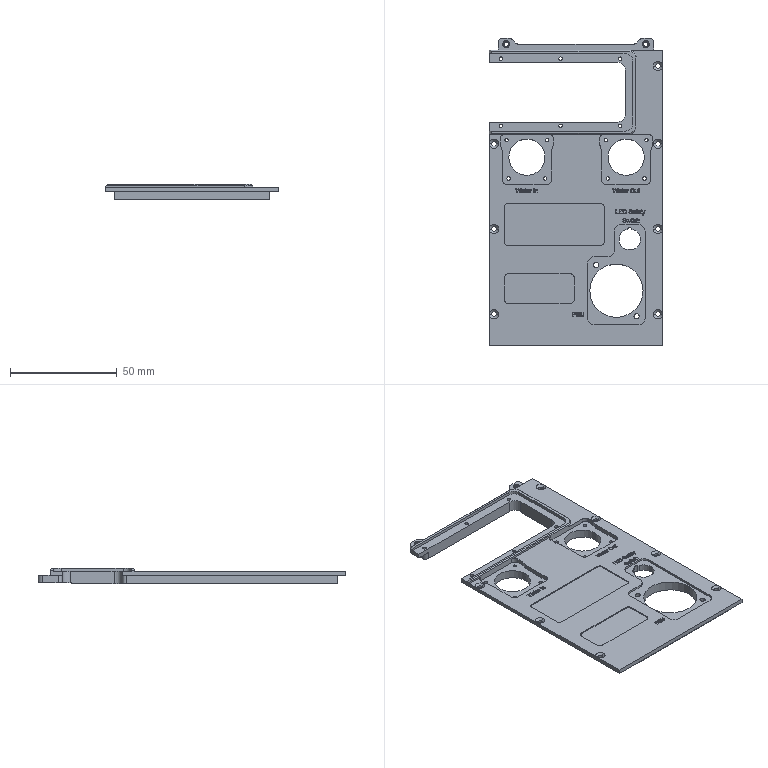NC program | NX | posted with a generic post | part box 81.5 x 144.28 x 7.5 mm
Lines 1 to 2085 of 3119, first 1845 of 2067 lines:
N10 G17 G21 G94 G90
(FLOOR_FACING_COPY , TOOL : D63面刀)
N12 T11 M6
N14 G54
N16 G17 G0 G90 X-113.64 Y25. S4500 M3
N18 G43 Z50. H11
N20 Z5.275
N22 G94 G1 Z2.275 F800.
N24 X-103.64
N26 X103.64
N28 Y-15.55
N30 X-103.64
N32 X-113.64
N34 Z5.275
N36 G0 Z50.
N38 Y25.
N40 Z4.55
N42 G1 Z1.55
N44 X-103.64
N46 X103.64
N48 Y-15.55
N50 X-103.64
N52 X-113.64
N54 Z4.55
N56 G0 Z50.
N58 Y25.
N60 Z3.825
N62 G1 Z0.825
N64 X-103.64
N66 X103.64
N68 Y-15.55
N70 X-103.64
N72 X-113.64
N74 Z3.825
N76 G0 Z50.
N78 Y25.
N80 Z3.1
N82 G1 Z0.1
N84 X-103.64
N86 X103.64
N88 Y-15.55
N90 X-103.64
N92 X-113.64
N94 Z3.1
N96 G0 Z50.
N98 M5
(CAVITY_MILL_COPY_2 , TOOL : D6开粗)
N100 T01 M6
N102 G54
N104 G17 G0 G90 X21.572 Y-44.35 S6500 M3
N106 G43 Z50. H1
N108 Z0.05
N110 G94 G1 Z-0.45 F2500.
N112 Y-41.65
N114 G3 X20.972 Y-41.05 R0.6
N116 G1 X-22.953 Y-41.049
N118 G2 X-24.802 Y-43.749 R4.206
N120 G1 X-30.848
N122 G2 X-32.725 Y-41.049 R4.261
N124 G1 X-60.964
N126 G2 X-62.725 Y-43.685 R4.381
N128 G1 X-62.819 Y-43.749
N130 X-66.705
N132 X-67.549 Y-43.692
N134 G2 X-69.926 Y-41.239 R3.002
N136 G3 X-70.169 Y-39.58 R7.304
N138 G1 X-70.227 Y-39.556
N140 X-70.811 Y-39.445
N142 Y-36.682
N144 G2 X-72.431 Y-34.455 R2.316
N146 X-72.419 Y-31.238 R70.632
N148 X-71.731 Y-29.673 R2.406
N150 G1 X-70.811 Y-28.748
N152 Y24.55
N154 G2 X-70.082 Y27.936 R8.221
N156 G3 X-70.428 Y28.362 R2.7
N158 G1 X-71.535 Y29.471
N160 X-71.727 Y29.669
N162 G2 X-72.419 Y31.239 R2.413
N164 X-72.432 Y34.488 R72.577
N166 X-70.426 Y36.77 R2.318
N168 G1 X-69.721 Y36.903
N170 G3 X-69.004 Y37.144 R2.702
N172 X-67.542 Y38.925 R2.7
N174 X-67.244 Y40.807 R10.604
N176 G2 X-66.985 Y41.049 R0.26
N178 G1 X72.14 Y41.05
N180 G2 X72.439 Y40.751 R0.299
N182 G1 Y-40.752
N184 G2 X72.14 Y-41.05 R0.299
N186 G1 X20.972
N188 Y-35.65
N190 X-22.869 Y-35.649
N192 Y-29.641
N194 G3 X-22.869 Y-16.458 R-9.276
N196 G1 X-22.109 Y-17.226
N198 G2 X-22.869 Y-28.008 R-8.196
N200 G1 Y-18.092
N202 G2 X-22.109 Y-17.226 R8.196
N204 G1 X-22.869 Y-16.458
N206 Y16.96
N208 G3 X-24.023 Y28.75 R-9.276
N210 G1 X-23.128 Y28.145
N212 G2 X-22.869 Y18.595 R-8.196
N214 G1 Y24.55
N216 G3 X-23.46 Y27.612 R8.221
N218 G2 X-23.128 Y28.145 R8.196
N220 G1 X-24.023 Y28.75
N222 G3 X-31.09 Y32.771 R8.221
N224 G1 X-62.59
N226 G3 X-66.321 Y31.876 R8.221
N228 X-66.606 Y32.176 R8.1
N230 G1 X-66.693 Y32.264
N232 X-69.355 Y33.778
N234 X-66.693 Y32.264
N236 G3 X-63.08 Y35.649 R8.1
N238 G1 X67.039 Y35.65
N240 X69.249 Y37.86
N242 X67.039 Y35.65
N244 Y-35.65
N246 X69.248 Y-37.86
N248 X67.039 Y-35.65
N250 X20.972
N252 Y-30.25
N254 X-3.554
N256 X-6.942 Y-31.987
N258 X-3.554 Y-30.25
N260 G3 X-17.469 Y-8.417 R14.676
N262 G1 X-19.57 Y-10.872
N264 X-17.469 Y-8.417
N266 Y8.918
N268 X-19.57 Y11.373
N270 X-17.469 Y8.918
N272 G3 X-3.283 Y30.25 R14.676
N274 G1 X-6.557 Y32.019
N276 X-3.283 Y30.25
N278 X19.503
N280 X22.312 Y32.25
N282 X19.503 Y30.25
N284 G3 X17.516 Y28.418 R5.769
N286 X16.88 Y26.429 R3.78
N288 G1 X16.867 Y26.345
N290 G3 X16.819 Y24.325 R3.78
N292 G2 X16.898 Y23.818 R2.83
N294 G3 X17.554 Y21.926 R3.78
N296 X27.02 Y21.859 R5.769
N298 X27.704 Y23.769 R3.78
N300 G1 X27.731 Y24.134
N302 G3 X27.74 Y24.407 R3.78
N304 G1 Y26.14
N306 X27.737 Y26.378
N308 G3 X27.085 Y28.451 R3.78
N310 X25.121 Y30.25 R5.769
N312 G1 X24.595 Y29.306
N314 G2 X26.191 Y27.844 R4.689
N316 X26.657 Y26.364 R2.7
N318 G1 X26.66 Y26.09
N320 Y24.407
N322 X26.653 Y24.212
N324 X26.627 Y23.847
N326 G2 X26.138 Y22.483 R2.7
N328 X18.444 Y22.537 R4.689
N330 X17.976 Y23.889 R2.7
N332 G3 X17.866 Y24.589 R3.91
N334 G2 X17.9 Y26.031 R2.7
N336 G3 X17.96 Y26.397 R1.402
N338 G2 X18.414 Y27.817 R2.7
N340 X24.595 Y29.306 R4.689
N342 G1 X25.121 Y30.25
N344 X39.344
N346 X42.059 Y31.526
N348 G2 X50.562 Y31.526 R13.275
N350 X51.477 Y32.65 R3.
N352 G1 X41.144
N354 G2 X42.059 Y31.526 R3.
N356 G1 X39.344 Y30.25
N358 G3 X33.574 Y22.69 R13.275
N360 G1 X31.23 Y26.129
N362 X33.574 Y22.69
N364 G3 X53.277 Y30.25 R-13.275
N366 G1 X52.71 Y29.331
N368 G2 X56.691 Y12.551 R12.195
N370 X52.71 Y29.331 R-12.195
N372 G1 X53.277 Y30.25
N374 X61.639
N376 X63.849 Y32.46
N378 X61.639 Y30.25
N380 Y-30.25
N382 X63.848 Y-32.46
N384 X61.639 Y-30.25
N386 X20.972
N388 Y-24.85
N390 X3.653
N392 X1.216 Y-26.955
N394 X3.653 Y-24.85
N396 G3 X-12.069 Y-3.434 R20.076
N398 G1 X-14.396 Y-5.404
N400 X-12.069 Y-3.434
N402 Y3.935
N404 X-14.396 Y5.904
N406 X-12.069 Y3.935
N408 G3 X3.693 Y24.85 R20.076
N410 G1 X1.297 Y26.975
N412 X3.693 Y24.85
N414 X11.313
N416 X13.647 Y27.008
N418 X11.313 Y24.85
N420 G3 X11.528 Y23.233 R9.18
N422 X13.101 Y18.871 R9.18
N424 X27.948 Y15.549 R11.169
N426 G1 X29.471 Y19.188
N428 X27.948 Y15.549
N430 G3 X56.239 Y3.133 R18.675
N432 G1 X57.943 Y6.557
N434 X56.239 Y3.133
N436 Y-24.85
N438 X58.448 Y-27.06
N440 X56.239 Y-24.85
N442 X20.972
N444 Y-19.45
N446 X8.878
N448 X6.817 Y-21.735
N450 X8.878 Y-19.45
N452 G3 X-6.04 Y0.25 R25.476
N454 G1 X-8.938
N456 X-6.04
N458 G3 X8.161 Y16.575 R25.476
N460 G1 X7.736 Y20.542
N462 X8.161 Y16.575
N464 G3 X8.649 Y15.815 R14.58
N466 X24.496 Y8.766 R16.569
N468 G1 X25.927 Y11.44
N470 X24.496 Y8.766
N472 G3 X50.839 Y-4.695 R24.075
N474 G1 X52.871 Y-2.112
N476 X50.839 Y-4.695
N478 Y-19.45
N480 X53.048 Y-21.66
N482 X50.839 Y-19.45
N484 X20.972
N486 Y-14.05
N488 X13.193
N490 X11.367 Y-16.439
N492 X13.193 Y-14.05
N494 G3 X3.917 Y0.25 R30.876
N496 G1 X0.642
N498 X3.917
N500 G3 X9.805 Y7.128 R30.876
N502 G1 X9.183 Y10.284
N504 X9.805 Y7.128
N506 G3 X21.371 Y3.242 R21.969
N508 X45.439 Y-10.512 R29.475
N510 G1 X47.647 Y-8.291
N512 X45.439 Y-10.512
N514 Y-14.05
N516 X47.648 Y-16.26
N518 X45.439 Y-14.05
N520 X20.972
N522 Y-8.65
N524 X16.953
N526 G3 X11.7 Y-0.038 R36.276
N528 G1 X8.577 Y0.297
N530 X11.7 Y-0.038
N532 X10.675 Y2.882
N534 X11.7 Y-0.038
N536 G3 X18.347 Y-1.89 R27.369
N538 X24.992 Y-8.65 R34.875
N540 G1 X26.792 Y-11.05
N542 X33.876
N544 G2 X27.861 Y-7.775 R32.475
N546 X26.792 Y-11.05 R3.
N548 G1 X24.992 Y-8.65
N550 X20.972
N552 G3 X20.76 Y-8.738 R0.3
N554 G1 Z0.05
N556 G0 Z50.
N558 X-33.834 Y22.777
N560 Z0.5
N562 G2 X-33.834 Y22.777 Z0.164 I0.977 J-0.294
N564 X-33.834 Y22.777 Z-0.172 I0.977 J-0.294
N566 X-33.578 Y21.762 Z-0.45 R-1.02
N568 G1 X-34.337 Y22.52
N570 X-32.82
N572 Y21.003
N574 X-33.578 Y21.762
N576 G3 X-33.791 Y21.849 R0.3
N578 G1 Z0.05
N580 G0 Z0.5
N582 X-61.117 Y21.506
N584 G2 X-61.117 Y21.506 Z0.164 I0.294 J0.977
N586 X-61.117 Y21.506 Z-0.172 I0.294 J0.977
N588 X-60.102 Y21.762 Z-0.45 R-1.02
N590 G1 X-60.86 Y21.003
N592 X-60.096 Y20.239
N594 X-57.089 Y23.247
N596 X-36.591
N598 X-32.843 Y19.499
N600 Y-40.747
N602 X-60.837
N604 Y19.499
N606 X-60.096 Y20.239
N608 X-60.86 Y21.003
N610 Y22.52
N612 X-59.343
N614 Y23.6
N616 X-61.355
N618 G3 X-61.94 Y22.962 R0.601
N620 G1 Y-39.614
N622 Y-39.736
N624 Y-40.124
N626 G2 X-63.345 Y-42.801 R3.301
N628 X-65.041 Y-43.336 R2.952
N630 G1 X-66.598
N632 G2 X-69.731 Y-40.203 R3.133
N634 G1 Y24.55
N636 G2 X-62.59 Y31.691 R7.141
N638 G1 X-31.09
N640 G2 X-23.949 Y24.55 R7.141
N642 G1 Y-40.21
N644 G2 X-27.075 Y-43.336 R3.126
N646 G1 X-28.59
N648 G2 X-31.74 Y-40.124 R3.181
N650 G1 Y-39.736
N652 Y-39.614
N654 Y23.009
N656 G3 X-32.373 Y23.6 R0.601
N658 G1 X-59.343
N660 Y22.52
N662 X-60.102 Y21.762
N664 G3 X-60.102 Y20.913 R0.6
N666 G1 Z0.05
N668 G0 Z50.
N670 X21.572 Y-44.35
N672 Z-0.4
N674 G1 Z-0.9
N676 Y-41.65
N678 G3 X20.972 Y-41.05 R0.6
N680 G1 X-22.883
N682 G2 X-24.245 Y-43.75 R4.261
N684 G1 X-26.637
N686 G3 X-23.94 Y-40.574 R3.181
N688 G1 Y24.55
N690 G3 X-31.09 Y31.7 R7.15
N692 G1 X-62.59
N694 G3 X-69.74 Y24.55 R7.15
N696 G1 Y-40.323
N698 X-69.741 Y-40.574
N700 G3 X-67.23 Y-43.714 R3.189
N702 G1 X-67.549 Y-43.692
N704 G2 X-69.926 Y-41.239 R3.002
N706 G3 X-70.169 Y-39.58 R7.299
N708 G1 X-70.227 Y-39.556
N710 X-70.82 Y-39.443
N712 Y-36.679
N714 G2 X-72.432 Y-34.456 R2.317
N716 X-72.419 Y-31.238 R72.082
N718 X-71.731 Y-29.673 R2.408
N720 G1 X-70.82 Y-28.756
N722 Y24.55
N724 G2 X-70.088 Y27.944 R8.23
N726 G3 X-70.428 Y28.362 R2.7
N728 G1 X-71.535 Y29.471
N730 X-71.728 Y29.67
N732 G2 X-72.419 Y31.239 R2.411
N734 X-72.432 Y34.488 R71.77
N736 X-70.425 Y36.77 R2.317
N738 G1 X-69.722 Y36.903
N740 G3 X-69.068 Y37.115 R2.701
N742 X-67.542 Y38.925 R2.7
N744 X-67.244 Y40.807 R10.601
N746 G2 X-66.985 Y41.049 R0.26
N748 G1 X72.14 Y41.05
N750 G2 X72.439 Y40.751 R0.299
N752 G1 Y-40.752
N754 G2 X72.14 Y-41.05 R0.299
N756 G1 X20.972
N758 Y-35.65
N760 X-18.54
N762 X-20.75 Y-37.859
N764 X-18.54 Y-35.65
N766 Y-32.061
N768 G3 X-18.54 Y-14.038 R-9.276
N770 G1 X-18.284 Y-15.087
N772 G2 X-22.86 Y-28.018 R-8.196
N774 G1 Y-18.081
N776 G2 X-18.284 Y-15.087 R8.196
N778 G1 X-18.54 Y-14.038
N780 Y14.539
N782 G3 X-20.775 Y31.698 R-9.276
N784 G1 X-20.259 Y30.75
N786 G2 X-22.86 Y18.583 R-8.196
N788 G1 Y24.55
N790 G3 X-23.455 Y27.621 R8.23
N792 G2 X-20.259 Y30.75 R8.196
N794 G1 X-20.775 Y31.698
N796 G3 X-25.233 Y35.65 R12.55
N798 G1 X-27.033 Y38.05
N800 X-64.67 Y38.049
N802 G2 X-67.854 Y34.371 R5.7
N804 X-69.164 Y33.955 R5.7
N806 G1 X-69.44 Y33.903
N808 G3 X-69.436 Y32.044 R68.77
N810 G2 X-62.59 Y34.7 R10.15
N812 G1 X-31.09
N814 G2 X-27.841 Y34.166 R10.15
N816 X-27.033 Y38.05 R3.
N818 G1 X-25.233 Y35.65
N820 X67.039
N822 X69.249 Y37.86
N824 X67.039 Y35.65
N826 Y-35.65
N828 X69.248 Y-37.86
N830 X67.039 Y-35.65
N832 X20.972
N834 Y-30.25
N836 X-3.554
N838 X-6.942 Y-31.987
N840 X-3.554 Y-30.25
N842 G3 X-13.14 Y-8.728 R14.676
N844 G1 X-15.459 Y-10.717
N846 X-13.14 Y-8.728
N848 Y9.228
N850 X-15.459 Y11.218
N852 X-13.14 Y9.228
N854 G3 X-3.283 Y30.25 R14.676
N856 G1 X-6.557 Y32.019
N858 X-3.283 Y30.25
N860 X19.504
N862 X22.312 Y32.25
N864 X19.504 Y30.25
N866 G3 X17.517 Y28.419 R5.769
N868 X16.88 Y26.428 R3.78
N870 G1 X16.867 Y26.343
N872 G3 X16.819 Y24.327 R3.78
N874 G2 X16.898 Y23.819 R2.852
N876 G3 X17.554 Y21.926 R3.78
N878 X27.02 Y21.859 R5.769
N880 X27.704 Y23.769 R3.78
N882 G1 X27.731 Y24.134
N884 G3 X27.74 Y24.408 R3.78
N886 G1 Y26.136
N888 X27.737 Y26.373
N890 G3 X27.084 Y28.452 R3.78
N892 X25.12 Y30.25 R5.769
N894 G1 X24.594 Y29.306
N896 G2 X26.191 Y27.845 R4.689
N898 X26.657 Y26.36 R2.7
N900 G1 X26.66 Y26.091
N902 Y24.407
N904 X26.653 Y24.212
N906 X26.627 Y23.847
N908 G2 X26.138 Y22.483 R2.7
N910 X18.444 Y22.537 R4.689
N912 X17.976 Y23.889 R2.7
N914 G3 X17.866 Y24.591 R3.932
N916 G2 X17.9 Y26.03 R2.7
N918 G3 X17.96 Y26.396 R1.407
N920 G2 X18.415 Y27.818 R2.7
N922 X24.594 Y29.306 R4.689
N924 G1 X25.12 Y30.25
N926 X39.345
N928 X42.06 Y31.526
N930 G2 X50.561 Y31.526 R13.275
N932 X51.476 Y32.65 R3.
N934 G1 X41.145
N936 G2 X42.06 Y31.526 R3.
N938 G1 X39.345 Y30.25
N940 G3 X33.574 Y22.689 R13.275
N942 G1 X31.231 Y26.129
N944 X33.574 Y22.689
N946 G3 X53.276 Y30.25 R-13.275
N948 G1 X52.71 Y29.331
N950 G2 X56.691 Y12.551 R12.195
N952 X52.71 Y29.331 R-12.195
N954 G1 X53.276 Y30.25
N956 X61.639
N958 X63.849 Y32.46
N960 X61.639 Y30.25
N962 Y-30.25
N964 X63.848 Y-32.46
N966 X61.639 Y-30.25
N968 X20.972
N970 Y-24.85
N972 X3.652
N974 X1.216 Y-26.955
N976 X3.652 Y-24.85
N978 G3 X-7.74 Y-4.91 R20.076
N980 G1 Y5.411
N982 G3 X3.693 Y24.85 R20.076
N984 G1 X1.297 Y26.975
N986 X3.693 Y24.85
N988 X11.313
N990 X13.647 Y27.008
N992 X11.313 Y24.85
N994 G3 X11.528 Y23.236 R9.18
N996 X13.101 Y18.871 R9.18
N998 X27.948 Y15.549 R11.169
N1000 G1 X29.471 Y19.189
N1002 X27.948 Y15.549
N1004 G3 X56.239 Y3.133 R18.675
N1006 G1 X57.943 Y6.557
N1008 X56.239 Y3.133
N1010 Y-24.85
N1012 X58.448 Y-27.06
N1014 X56.239 Y-24.85
N1016 X20.972
N1018 Y-19.45
N1020 X8.878
N1022 X6.817 Y-21.735
N1024 X8.878 Y-19.45
N1026 G3 X-2.34 Y-1.767 R25.476
N1028 G1 Y2.267
N1030 G3 X8.161 Y16.575 R25.476
N1032 G1 X7.736 Y20.542
N1034 X8.161 Y16.575
N1036 G3 X8.649 Y15.815 R14.58
N1038 X24.496 Y8.766 R16.569
N1040 G1 X25.927 Y11.44
N1042 X24.496 Y8.766
N1044 G3 X50.839 Y-4.695 R24.075
N1046 G1 X52.871 Y-2.112
N1048 X50.839 Y-4.695
N1050 Y-19.45
N1052 X53.048 Y-21.66
N1054 X50.839 Y-19.45
N1056 X20.972
N1058 Y-14.05
N1060 X13.193
N1062 X11.367 Y-16.439
N1064 X13.193 Y-14.05
N1066 G3 X3.917 Y0.25 R30.876
N1068 G1 X0.812
N1070 X3.917
N1072 G3 X9.805 Y7.128 R30.876
N1074 G1 X9.183 Y10.284
N1076 X9.805 Y7.128
N1078 G3 X21.371 Y3.242 R21.969
N1080 X45.439 Y-10.512 R29.475
N1082 G1 X47.647 Y-8.291
N1084 X45.439 Y-10.512
N1086 Y-14.05
N1088 X47.648 Y-16.26
N1090 X45.439 Y-14.05
N1092 X20.972
N1094 Y-8.65
N1096 X16.953
N1098 G3 X11.701 Y-0.038 R36.276
N1100 G1 X10.674 Y2.882
N1102 X11.701 Y-0.038
N1104 X8.577 Y0.297
N1106 X11.701 Y-0.038
N1108 G3 X18.348 Y-1.89 R27.369
N1110 X24.992 Y-8.65 R34.875
N1112 G1 X26.792 Y-11.05
N1114 X33.877
N1116 G2 X27.862 Y-7.775 R32.475
N1118 X26.792 Y-11.05 R3.
N1120 G1 X24.992 Y-8.65
N1122 X20.972
N1124 G3 X20.76 Y-8.738 R0.3
N1126 G1 Z-0.4
N1128 G0 Z0.05
N1130 X21.572 Y-44.35
N1132 Z-0.85
N1134 G1 Z-1.35
N1136 X21.573 Y-41.65
N1138 G3 X20.973 Y-41.05 R0.6
N1140 G1 X-22.871
N1142 G2 X-24.108 Y-43.75 R4.23
N1144 G1 X-26.128
N1146 G3 X-23.94 Y-40.75 R3.15
N1148 G1 Y24.55
N1150 G3 X-31.09 Y31.7 R7.15
N1152 G1 X-62.59
N1154 G3 X-69.74 Y24.55 R7.15
N1156 G1 Y-40.323
N1158 Y-40.75
N1160 G3 X-68.012 Y-43.561 R3.15
N1162 G2 X-69.926 Y-41.239 R3.002
N1164 G3 X-70.169 Y-39.58 R7.294
N1166 G1 X-70.227 Y-39.556
N1168 X-70.82 Y-39.443
N1170 Y-36.679
N1172 G2 X-72.432 Y-34.458 R2.318
N1174 X-72.419 Y-31.238 R73.869
N1176 X-71.731 Y-29.673 R2.409
N1178 G1 X-70.82 Y-28.756
N1180 Y24.55
N1182 G2 X-70.088 Y27.944 R8.23
N1184 G3 X-70.428 Y28.362 R2.7
N1186 G1 X-71.535 Y29.471
N1188 X-71.727 Y29.669
N1190 G2 X-72.419 Y31.24 R2.417
N1192 X-72.432 Y34.488 R71.697
N1194 X-70.423 Y36.77 R2.318
N1196 G1 X-69.723 Y36.903
N1198 G3 X-69.098 Y37.101 R2.701
N1200 X-67.542 Y38.925 R2.7
N1202 X-67.244 Y40.807 R10.598
N1204 G2 X-66.985 Y41.049 R0.26
N1206 G1 X72.14 Y41.05
N1208 G2 X72.439 Y40.751 R0.299
N1210 G1 Y-40.752
N1212 G2 X72.14 Y-41.05 R0.299
N1214 G1 X20.973
N1216 Y-35.65
N1218 X-18.54
N1220 X-20.75 Y-37.859
N1222 X-18.54 Y-35.65
N1224 Y-32.061
N1226 G3 X-18.54 Y-14.038 R-9.276
N1228 G1 X-18.284 Y-15.087
N1230 G2 X-22.86 Y-28.018 R-8.196
N1232 G1 Y-18.081
N1234 G2 X-18.284 Y-15.087 R8.196
N1236 G1 X-18.54 Y-14.038
N1238 Y14.539
N1240 G3 X-20.775 Y31.698 R-9.276
N1242 G1 X-20.259 Y30.75
N1244 G2 X-22.86 Y18.583 R-8.196
N1246 G1 Y24.55
N1248 G3 X-23.455 Y27.621 R8.23
N1250 G2 X-20.259 Y30.75 R8.196
N1252 G1 X-20.775 Y31.698
N1254 G3 X-25.233 Y35.65 R12.55
N1256 G1 X-27.033 Y38.05
N1258 X-64.67 Y38.049
N1260 G2 X-67.919 Y34.343 R5.7
N1262 X-69.164 Y33.956 R5.7
N1264 G1 X-69.44 Y33.903
N1266 G3 X-69.436 Y32.044 R68.697
N1268 G2 X-62.59 Y34.7 R10.15
N1270 G1 X-31.09
N1272 G2 X-27.841 Y34.166 R10.15
N1274 X-27.033 Y38.05 R3.
N1276 G1 X-25.233 Y35.65
N1278 X67.039
N1280 X69.249 Y37.86
N1282 X67.039 Y35.65
N1284 Y-35.65
N1286 X69.248 Y-37.86
N1288 X67.039 Y-35.65
N1290 X20.973
N1292 Y-30.25
N1294 X-3.554
N1296 X-6.942 Y-31.987
N1298 X-3.554 Y-30.25
N1300 G3 X-13.14 Y-8.728 R14.676
N1302 G1 X-15.459 Y-10.717
N1304 X-13.14 Y-8.728
N1306 Y9.228
N1308 X-15.459 Y11.218
N1310 X-13.14 Y9.228
N1312 G3 X-3.283 Y30.25 R14.676
N1314 G1 X-6.557 Y32.019
N1316 X-3.283 Y30.25
N1318 X19.504
N1320 X22.312 Y32.25
N1322 X19.504 Y30.25
N1324 G3 X17.517 Y28.419 R5.769
N1326 X16.88 Y26.427 R3.78
N1328 G1 X16.866 Y26.34
N1330 G3 X16.818 Y24.33 R3.78
N1332 G2 X16.898 Y23.819 R2.875
N1334 G3 X17.554 Y21.926 R3.78
N1336 X27.02 Y21.859 R5.769
N1338 X27.704 Y23.769 R3.78
N1340 G1 X27.731 Y24.134
N1342 G3 X27.74 Y24.408 R3.78
N1344 G1 Y26.131
N1346 X27.737 Y26.369
N1348 G3 X27.084 Y28.452 R3.78
N1350 X25.12 Y30.25 R5.769
N1352 G1 X24.594 Y29.306
N1354 G2 X26.191 Y27.845 R4.689
N1356 X26.657 Y26.357 R2.7
N1358 G1 X26.66 Y26.091
N1360 Y24.408
N1362 X26.653 Y24.212
N1364 X26.627 Y23.847
N1366 G2 X26.138 Y22.483 R2.7
N1368 X18.444 Y22.537 R4.689
N1370 X17.976 Y23.889 R2.7
N1372 G3 X17.866 Y24.592 R3.955
N1374 G2 X17.9 Y26.028 R2.7
N1376 G3 X17.96 Y26.395 R1.412
N1378 G2 X18.415 Y27.818 R2.7
N1380 X24.594 Y29.306 R4.689
N1382 G1 X25.12 Y30.25
N1384 X39.345
N1386 X42.06 Y31.526
N1388 G2 X50.561 Y31.526 R13.274
N1390 X51.476 Y32.65 R3.
N1392 G1 X41.145
N1394 G2 X42.06 Y31.526 R3.
N1396 G1 X39.345 Y30.25
N1398 G3 X33.574 Y22.688 R13.274
N1400 G1 X31.231 Y26.129
N1402 X33.574 Y22.688
N1404 G3 X53.276 Y30.25 R-13.274
N1406 G1 X52.71 Y29.331
N1408 G2 X56.692 Y12.551 R12.194
N1410 X52.71 Y29.331 R-12.194
N1412 G1 X53.276 Y30.25
N1414 X61.639
N1416 X63.849 Y32.46
N1418 X61.639 Y30.25
N1420 Y-30.25
N1422 X63.848 Y-32.46
N1424 X61.639 Y-30.25
N1426 X20.973
N1428 Y-24.85
N1430 X3.652
N1432 X1.216 Y-26.955
N1434 X3.652 Y-24.85
N1436 G3 X-7.74 Y-4.91 R20.076
N1438 G1 Y5.411
N1440 G3 X3.693 Y24.85 R20.076
N1442 G1 X1.297 Y26.975
N1444 X3.693 Y24.85
N1446 X11.314
N1448 X13.647 Y27.008
N1450 X11.314 Y24.85
N1452 G3 X11.528 Y23.24 R9.18
N1454 X13.101 Y18.871 R9.18
N1456 X27.949 Y15.549 R11.169
N1458 G1 X29.471 Y19.189
N1460 X27.949 Y15.549
N1462 G3 X56.239 Y3.133 R18.674
N1464 G1 X57.943 Y6.558
N1466 X56.239 Y3.133
N1468 Y-24.85
N1470 X58.449 Y-27.06
N1472 X56.239 Y-24.85
N1474 X20.973
N1476 Y-19.45
N1478 X8.878
N1480 X6.817 Y-21.735
N1482 X8.878 Y-19.45
N1484 G3 X-2.34 Y-1.767 R25.476
N1486 G1 Y2.267
N1488 G3 X8.161 Y16.575 R25.476
N1490 G1 X7.736 Y20.542
N1492 X8.161 Y16.575
N1494 G3 X8.649 Y15.815 R14.58
N1496 X24.496 Y8.766 R16.569
N1498 G1 X25.927 Y11.44
N1500 X24.496 Y8.766
N1502 G3 X50.839 Y-4.695 R24.074
N1504 G1 X52.871 Y-2.112
N1506 X50.839 Y-4.695
N1508 Y-19.45
N1510 X53.049 Y-21.66
N1512 X50.839 Y-19.45
N1514 X20.973
N1516 Y-14.05
N1518 X13.193
N1520 X11.367 Y-16.439
N1522 X13.193 Y-14.05
N1524 G3 X3.917 Y0.25 R30.876
N1526 G1 X0.812
N1528 X3.917
N1530 G3 X9.805 Y7.128 R30.876
N1532 G1 X9.183 Y10.284
N1534 X9.805 Y7.128
N1536 G3 X21.371 Y3.242 R21.969
N1538 X45.439 Y-10.512 R29.474
N1540 G1 X47.647 Y-8.291
N1542 X45.439 Y-10.512
N1544 Y-14.05
N1546 X47.649 Y-16.26
N1548 X45.439 Y-14.05
N1550 X20.973
N1552 Y-8.65
N1554 X16.953
N1556 G3 X11.701 Y-0.038 R36.276
N1558 G1 X10.674 Y2.882
N1560 X11.701 Y-0.038
N1562 X8.577 Y0.297
N1564 X11.701 Y-0.038
N1566 G3 X18.348 Y-1.89 R27.369
N1568 X24.992 Y-8.65 R34.874
N1570 G1 X26.792 Y-11.05
N1572 X33.877
N1574 G2 X27.862 Y-7.775 R32.474
N1576 X26.792 Y-11.05 R3.
N1578 G1 X24.992 Y-8.65
N1580 X20.973
N1582 G3 X20.761 Y-8.738 R0.3
N1584 G1 Z-0.85
N1586 G0 Z-0.4
N1588 X33.425 Y24.611
N1590 Z-0.85
N1592 G2 X31.593 Y29.295 Z-1.4 R-2.7
N1594 G1 X59.155
N1596 Y8.605
N1598 X33.465
N1600 Y15.
N1602 G3 X27.36 Y21.105 R6.105
N1604 G1 X18.415
N1606 Y29.295
N1608 X31.593
N1610 Y26.595
N1612 X35.459
N1614 G3 X33.286 Y21.512 R13.274
N1616 G1 X34.346 Y21.303
N1618 G2 X38.383 Y28.215 R12.194
N1620 G1 X44.238
N1622 G2 X48.384 Y28.215 R9.494
N1624 G1 X54.239
N1626 G2 X58.075 Y22.159 R12.194
N1628 G1 Y15.741
N1630 G2 X54.239 Y9.685 R12.194
N1632 G1 X48.384
N1634 G2 X44.238 Y9.685 R9.494
N1636 G1 X38.383
N1638 G2 X34.469 Y16.037 R12.194
N1640 G3 X34.292 Y16.889 R7.185
N1642 G2 X34.346 Y21.303 R12.194
N1644 G1 X33.286 Y21.512
N1646 G3 X27.706 Y23.798 R8.805
N1648 G1 X27.731 Y24.134
N1650 G3 X27.74 Y24.408 R3.78
N1652 G1 X27.739 Y26.13
N1654 X27.737 Y26.368
N1656 G3 X27.728 Y26.595 R3.78
N1658 G1 X26.65 Y26.519
N1660 X26.657 Y26.357
N1662 X26.66 Y26.091
N1664 Y24.408
N1666 X26.653 Y24.212
N1668 X26.627 Y23.847
N1670 G2 X26.138 Y22.483 R2.7
N1672 X25.909 Y22.185 R4.689
N1674 G1 X19.495
N1676 Y28.215
N1678 X25.911
N1680 G2 X26.191 Y27.845 R4.689
N1682 X26.65 Y26.519 R2.7
N1684 G1 X27.728 Y26.595
N1686 X31.593
N1688 G3 X32.193 Y27.195 R0.6
N1690 G1 Z-0.9
N1692 G0 Z-0.85
N1694 X30.467 Y29.003
N1696 Z-0.9
N1698 G2 X30.467 Y29.003 Z-1.789 I1.129 J-2.453
N1700 X31.593 Y29.25 Z-1.85 R2.7
N1702 G1 X59.11
N1704 Y8.65
N1706 X33.51
N1708 Y15.
N1710 G3 X27.36 Y21.15 R6.15
N1712 G1 X18.46
N1714 Y29.25
N1716 X31.593
N1718 Y26.55
N1720 X35.428
N1722 G3 X33.296 Y21.564 R13.274
N1724 G1 X34.355 Y21.351
N1726 G2 X38.33 Y28.17 R12.194
N1728 G1 X44.045
N1730 G2 X48.577 Y28.17 R9.494
N1732 G1 X54.292
N1734 G2 X58.03 Y22.321 R12.194
N1736 G1 Y15.579
N1738 G2 X54.292 Y9.73 R12.194
N1740 G1 X48.577
N1742 G2 X44.045 Y9.73 R9.494
N1744 G1 X38.33
N1746 G2 X34.555 Y15.709 R12.194
N1748 G3 X34.239 Y17.225 R7.23
N1750 G2 X34.355 Y21.351 R12.194
N1752 G1 X33.296 Y21.564
N1754 G3 X27.71 Y23.843 R8.85
N1756 G1 X27.731 Y24.134
N1758 G3 X27.74 Y24.413 R3.78
N1760 G1 X27.737 Y26.334
N1762 G3 X27.731 Y26.55 R3.78
N1764 G1 X26.652 Y26.487
N1766 X26.657 Y26.333
N1768 X26.66 Y24.411
N1770 X26.653 Y24.212
N1772 X26.627 Y23.847
N1774 G2 X26.138 Y22.483 R2.7
N1776 X25.946 Y22.23 R4.689
N1778 G1 X19.54
N1780 Y28.17
N1782 X25.949
N1784 G2 X26.191 Y27.845 R4.689
N1786 X26.652 Y26.487 R2.7
N1788 G1 X27.731 Y26.55
N1790 X31.593
N1792 G3 X32.193 Y27.15 R0.6
N1794 G1 Z-1.35
N1796 G0 Z-0.9
N1798 X29.688 Y28.46
N1800 Z-1.35
N1802 G2 X29.688 Y28.46 Z-2.239 I1.908 J-1.91
N1804 X31.593 Y29.25 Z-2.35 R2.7
N1806 G1 X59.11
N1808 Y8.65
N1810 X33.51
N1812 Y15.
N1814 G3 X27.36 Y21.15 R6.15
N1816 G1 X18.46
N1818 Y29.25
N1820 X31.593
N1822 Y26.55
N1824 X35.428
N1826 G3 X33.297 Y21.563 R13.274
N1828 G1 X34.355 Y21.351
N1830 G2 X38.33 Y28.17 R12.194
N1832 G1 X44.045
N1834 G2 X48.577 Y28.17 R9.494
N1836 G1 X54.292
N1838 G2 X58.03 Y22.321 R12.194
N1840 G1 Y15.579
N1842 G2 X54.292 Y9.73 R12.194
N1844 G1 X48.576
N1846 G2 X44.046 Y9.73 R9.494
N1848 G1 X38.33
N1850 G2 X34.555 Y15.71 R12.194
N1852 G3 X34.24 Y17.223 R7.23
N1854 G2 X34.355 Y21.351 R12.194
N1856 G1 X33.297 Y21.563
N1858 G3 X27.71 Y23.843 R8.85
N1860 G1 X27.731 Y24.134
N1862 G3 X27.74 Y24.413 R3.78
N1864 G1 X27.737 Y26.334
N1866 G3 X27.731 Y26.55 R3.78
N1868 G1 X26.652 Y26.487
N1870 X26.657 Y26.333
N1872 X26.66 Y24.411
N1874 X26.653 Y24.212
N1876 X26.627 Y23.847
N1878 G2 X26.138 Y22.483 R2.7
N1880 X25.946 Y22.23 R4.689
N1882 G1 X19.54
N1884 Y28.17
N1886 X25.949
N1888 G2 X26.191 Y27.845 R4.689
N1890 X26.652 Y26.487 R2.7
N1892 G1 X27.731 Y26.55
N1894 X31.593
N1896 G3 X32.193 Y27.15 R0.6
N1898 G1 Z-1.85
N1900 G0 Z50.
N1902 X44.521 Y-19.081
N1904 Z-0.85
N1906 G2 X49.205 Y-17.25 Z-1.4 R-2.7
N1908 G1 Y-30.645
N1910 X41.415
N1912 Y-3.855
N1914 X49.205
N1916 Y-17.25
N1918 X46.505
N1920 Y-27.945
N1922 X44.115
N1924 Y-6.555
N1926 X46.505
N1928 Y-17.25
N1930 G3 X47.105 Y-17.85 R0.6
N1932 G1 Z-0.9
N1934 G0 Z-0.85
N1936 X48.914 Y-16.123
N1938 Z-0.9
N1940 G2 X48.914 Y-16.123 Z-1.789 I-2.454 J-1.127
N1942 X49.16 Y-17.25 Z-1.85 R2.7
N1944 G1 Y-30.6
N1946 X41.46
N1948 Y-3.9
N1950 X49.16
N1952 Y-17.25
N1954 X46.46
N1956 Y-27.9
N1958 X44.16
N1960 Y-6.6
N1962 X46.46
N1964 Y-17.25
N1966 G3 X47.06 Y-17.85 R0.6
N1968 G1 Z-1.35
N1970 G0 X17.521 Y-12.081 Z-0.85
N1972 G2 X22.205 Y-10.25 Z-1.4 R-2.7
N1974 G1 Y-30.645
N1976 X8.415
N1978 Y10.145
N1980 X22.205
N1982 Y-10.25
N1984 X16.805
N1986 Y-25.245
N1988 X19.015 Y-27.455
N1990 X16.805 Y-25.245
N1992 X13.815
N1994 X11.605 Y-27.455
N1996 X13.815 Y-25.245
N1998 Y4.745
N2000 X11.605 Y6.955
N2002 X13.815 Y4.745
N2004 X16.805
N2006 X19.015 Y6.955
N2008 X16.805 Y4.745
N2010 Y-10.25
N2012 G3 X17.405 Y-10.85 R0.6
N2014 G1 Z-0.9
N2016 G0 Z-0.85
N2018 X21.914 Y-9.123
N2020 Z-0.9
N2022 G2 X21.914 Y-9.123 Z-1.789 I-2.454 J-1.127
N2024 X22.16 Y-10.25 Z-1.85 R2.7
N2026 G1 Y-30.6
N2028 X8.46
N2030 Y10.1
N2032 X22.16
N2034 Y-10.25
N2036 X16.76
N2038 Y-25.2
N2040 X18.97 Y-27.41
N2042 X16.76 Y-25.2
N2044 X13.86
N2046 X11.65 Y-27.41
N2048 X13.86 Y-25.2
N2050 Y4.7
N2052 X11.65 Y6.91
N2054 X13.86 Y4.7
N2056 X16.76
N2058 X18.97 Y6.91
N2060 X16.76 Y4.7
N2062 Y-10.25
N2064 G3 X17.36 Y-10.85 R0.6
N2066 G1 Z-1.35
N2068 G0 X-21.238 Y-23.05 Z-0.9
N2070 G1 Z-1.4
N2072 X-23.94
N2074 Y-13.805
N2076 X-22.499
N2078 X-20.162 Y-14.431
N2080 G3 X-18.841 Y-14.605 R5.105
N2082 G1 X-6.695
N2084 Y-31.495
N2086 X-18.841
N2088 G3 X-20.162 Y-31.669 R5.105
N2090 G1 X-22.499 Y-32.295
N2092 X-23.94
N2094 Y-23.05
N2096 Z-0.9
N2098 G0 Z-0.85
N2100 X-21.237
N2102 Z-1.35
N2104 G1 Z-1.85
N2106 X-23.94
N2108 Y-13.85
N2110 X-22.505
N2112 X-20.174 Y-14.475
N2114 G3 X-18.841 Y-14.65 R5.15
N2116 G1 X-6.74
N2118 Y-31.45
N2120 X-18.841
N2122 G3 X-20.174 Y-31.625 R5.15
N2124 G1 X-22.505 Y-32.25
N2126 X-23.94
N2128 Y-23.05
N2130 Z-1.35
N2132 G0 Z-0.9
N2134 X-21.237
N2136 Z-1.85
N2138 G1 Z-2.35
N2140 X-23.94
N2142 Y-13.85
N2144 X-22.505
N2146 X-20.174 Y-14.475
N2148 G3 X-18.841 Y-14.65 R5.15
N2150 G1 X-6.74
N2152 Y-31.45
N2154 X-18.841
N2156 G3 X-20.174 Y-31.625 R5.15
N2158 G1 X-22.505 Y-32.25
N2160 X-23.94
N2162 Y-23.05
N2164 Z-1.85
N2166 G0 Z-1.35
N2168 X-21.237
N2170 Z-2.35
N2172 G1 Z-2.85
N2174 X-23.94
N2176 Y-13.85
N2178 X-22.505
N2180 X-20.174 Y-14.475
N2182 G3 X-18.841 Y-14.65 R5.15
N2184 G1 X-6.74
N2186 Y-31.45
N2188 X-18.841
N2190 G3 X-20.174 Y-31.625 R5.15
N2192 G1 X-22.505 Y-32.25
N2194 X-23.94
N2196 Y-23.05
N2198 Z-2.35
N2200 G0 Z-1.85
N2202 X-21.237
N2204 Z-2.85
N2206 G1 Z-3.35
N2208 X-23.94
N2210 Y-13.85
N2212 X-22.505
N2214 X-20.174 Y-14.475
N2216 G3 X-18.841 Y-14.65 R5.15
N2218 G1 X-6.74
N2220 Y-31.45
N2222 X-18.841
N2224 G3 X-20.174 Y-31.625 R5.15
N2226 G1 X-22.505 Y-32.25
N2228 X-23.94
N2230 Y-23.05
N2232 Z-2.85
N2234 G0 Z50.
N2236 X-21.237 Y23.551
N2238 Z-0.9
N2240 G1 Z-1.4
N2242 X-23.94
N2244 Y24.55
N2246 G3 X-23.985 Y25.354 R7.15
N2248 G1 Y32.795
N2250 X-22.499
N2252 X-20.162 Y32.169
N2254 G3 X-18.841 Y31.995 R5.105
N2256 G1 X-6.695
N2258 Y15.105
N2260 X-18.841
N2262 G3 X-20.162 Y14.931 R5.105
N2264 G1 X-22.499 Y14.305
N2266 X-23.94
N2268 Y23.551
N2270 Z-0.9
N2272 G0 Z-0.85
N2274 X-21.237
N2276 Z-1.35
N2278 G1 Z-1.85
N2280 X-23.94
N2282 Y32.75
N2284 X-22.505
N2286 X-20.174 Y32.125
N2288 G3 X-18.841 Y31.95 R5.15
N2290 G1 X-6.74
N2292 Y15.15
N2294 X-18.841
N2296 G3 X-20.174 Y14.975 R5.15
N2298 G1 X-22.505 Y14.35
N2300 X-23.94
N2302 Y23.551
N2304 Z-1.35
N2306 G0 Z-0.9
N2308 X-21.237
N2310 Z-1.85
N2312 G1 Z-2.35
N2314 X-23.94
N2316 Y32.75
N2318 X-22.505
N2320 X-20.174 Y32.125
N2322 G3 X-18.841 Y31.95 R5.15
N2324 G1 X-6.74
N2326 Y15.15
N2328 X-18.841
N2330 G3 X-20.174 Y14.975 R5.15
N2332 G1 X-22.505 Y14.35
N2334 X-23.94
N2336 Y23.551
N2338 Z-1.85
N2340 G0 Z-1.35
N2342 X-21.237
N2344 Z-2.35
N2346 G1 Z-2.85
N2348 X-23.94
N2350 Y32.75
N2352 X-22.505
N2354 X-20.174 Y32.125
N2356 G3 X-18.841 Y31.95 R5.15
N2358 G1 X-6.74
N2360 Y15.15
N2362 X-18.841
N2364 G3 X-20.174 Y14.975 R5.15
N2366 G1 X-22.505 Y14.35
N2368 X-23.94
N2370 Y23.551
N2372 Z-2.35
N2374 G0 Z-1.85
N2376 X-21.237
N2378 Z-2.85
N2380 G1 Z-3.35
N2382 X-23.94
N2384 Y32.75
N2386 X-22.505
N2388 X-20.174 Y32.125
N2390 G3 X-18.841 Y31.95 R5.15
N2392 G1 X-6.74
N2394 Y15.15
N2396 X-18.841
N2398 G3 X-20.174 Y14.975 R5.15
N2400 G1 X-22.505 Y14.35
N2402 X-23.94
N2404 Y23.551
N2406 Z-2.85
N2408 G0 Z50.
N2410 X-72.94 Y-0.623
N2412 Z-0.9
N2414 G1 Z-1.4
N2416 X-71.42
N2418 G3 X-70.82 Y-0.023 R0.6
N2420 G1 Y24.55
N2422 G2 X-70.775 Y25.413 R8.23
N2424 G1 Y28.709
N2426 X-71.535 Y29.471
N2428 X-71.727 Y29.669
N2430 G2 X-72.42 Y31.24 R2.417
N2432 X-72.432 Y34.488 R71.733
N2434 X-70.775 Y36.693 R2.316
N2436 G1 Y39.452
N2438 X-70.226 Y39.556
N2440 X-70.16 Y39.584
N2442 G3 X-69.938 Y40.987 R7.897
N2444 G2 X-67.604 Y43.684 R2.96
N2446 G3 X-69.695 Y40.749 R3.106
N2448 G1 Y25.354
N2450 G3 X-69.74 Y24.55 R7.15
N2452 G1 Y-40.323
N2454 Y-40.75
N2456 G3 X-68.012 Y-43.561 R3.15
N2458 G2 X-69.926 Y-41.239 R3.002
N2460 G3 X-70.169 Y-39.58 R7.295
N2462 G1 X-70.227 Y-39.556
N2464 X-70.82 Y-39.443
N2466 Y-36.679
N2468 G2 X-72.432 Y-34.458 R2.318
N2470 X-72.419 Y-31.238 R73.894
N2472 X-71.731 Y-29.673 R2.409
N2474 G1 X-70.82 Y-28.756
N2476 Y-0.023
N2478 G3 X-71.42 Y0.577 R0.6
N2480 G1 X-72.94
N2482 Z-0.9
N2484 G0 Z-0.85
N2486 Y-0.601
N2488 Z-1.35
N2490 G1 Z-1.85
N2492 X-71.42
N2494 G3 X-70.82 Y-0.001 R0.6
N2496 G1 Y28.754
N2498 X-71.535 Y29.471
N2500 X-71.727 Y29.669
N2502 G2 X-72.42 Y31.239 R2.416
N2504 X-72.432 Y34.488 R72.054
N2506 X-70.82 Y36.679 R2.316
N2508 G1 Y39.443
N2510 X-70.228 Y39.556
N2512 X-70.16 Y39.584
N2514 G3 X-69.939 Y40.986 R7.894
N2516 G2 X-67.974 Y43.579 R2.96
N2518 G3 X-69.74 Y40.75 R3.15
N2520 G1 Y-40.323
N2522 Y-40.75
N2524 G3 X-68.011 Y-43.561 R3.15
N2526 G2 X-69.926 Y-41.239 R3.002
N2528 G3 X-70.169 Y-39.58 R7.303
N2530 G1 X-70.227 Y-39.556
N2532 X-70.82 Y-39.443
N2534 Y-36.679
N2536 G2 X-72.432 Y-34.458 R2.318
N2538 X-72.42 Y-31.238 R74.128
N2540 X-71.731 Y-29.673 R2.41
N2542 G1 X-70.82 Y-28.756
N2544 Y-0.001
N2546 G3 X-71.42 Y0.599 R0.6
N2548 G1 X-72.94
N2550 Z-1.35
N2552 G0 Z-0.9
N2554 Y-0.601
N2556 Z-1.85
N2558 G1 Z-2.35
N2560 X-71.42
N2562 G3 X-70.82 Y-0.001 R0.6
N2564 G1 Y28.754
N2566 X-71.535 Y29.471
N2568 X-71.728 Y29.669
N2570 G2 X-72.42 Y31.239 R2.414
N2572 X-72.432 Y34.488 R72.415
N2574 X-70.82 Y36.679 R2.316
N2576 G1 Y39.443
N2578 X-70.228 Y39.556
N2580 X-70.16 Y39.584
N2582 G3 X-69.939 Y40.986 R7.893
N2584 G2 X-67.973 Y43.58 R2.96
N2586 G3 X-69.74 Y40.75 R3.15
N2588 G1 Y-40.323
N2590 Y-40.75
N2592 G3 X-68.034 Y-43.549 R3.15
N2594 G2 X-69.936 Y-41.014 R2.881
N2596 G3 X-70.169 Y-39.58 R7.313
N2598 G1 X-70.227 Y-39.556
N2600 X-70.82 Y-39.443
N2602 Y-36.679
N2604 G2 X-72.432 Y-34.458 R2.318
N2606 X-72.42 Y-31.238 R74.389
N2608 X-71.731 Y-29.673 R2.412
N2610 G1 X-70.82 Y-28.756
N2612 Y-0.001
N2614 G3 X-71.42 Y0.599 R0.6
N2616 G1 X-72.94
N2618 Z-1.85
N2620 G0 Z-1.35
N2622 Y-0.601
N2624 Z-2.35
N2626 G1 Z-2.85
N2628 X-71.42
N2630 G3 X-70.82 Y-0.001 R0.6
N2632 G1 Y28.754
N2634 X-71.535 Y29.471
N2636 X-71.728 Y29.67
N2638 G2 X-72.42 Y31.239 R2.412
N2640 X-72.432 Y34.488 R72.779
N2642 X-70.82 Y36.679 R2.316
N2644 G1 Y39.443
N2646 X-70.228 Y39.556
N2648 X-70.16 Y39.584
N2650 G3 X-69.939 Y40.986 R7.889
N2652 G2 X-67.972 Y43.581 R2.96
N2654 G3 X-69.74 Y40.75 R3.15
N2656 G1 Y-40.323
N2658 Y-40.75
N2660 G3 X-68.033 Y-43.55 R3.15
N2662 G2 X-69.936 Y-41.015 R2.881
N2664 G3 X-70.169 Y-39.58 R7.322
N2666 G1 X-70.227 Y-39.556
N2668 X-70.82 Y-39.443
N2670 Y-36.679
N2672 G2 X-72.432 Y-34.458 R2.318
N2674 X-72.42 Y-31.238 R74.652
N2676 X-71.731 Y-29.673 R2.413
N2678 G1 X-70.82 Y-28.756
N2680 Y-0.001
N2682 G3 X-71.42 Y0.599 R0.6
N2684 G1 X-72.94
N2686 Z-2.35
N2688 G0 Z-1.85
N2690 X-72.941 Y-0.602
N2692 Z-2.85
N2694 G1 Z-3.35
N2696 X-71.42
N2698 G3 X-70.82 Y-0.002 R0.6
N2700 G1 Y28.753
N2702 X-71.534 Y29.47
N2704 X-71.727 Y29.669
N2706 G2 X-72.42 Y31.239 R2.419
N2708 X-72.432 Y34.488 R73.147
N2710 X-70.82 Y36.68 R2.317
N2712 G1 Y39.443
N2714 X-70.228 Y39.556
N2716 X-70.16 Y39.584
N2718 G3 X-69.939 Y40.986 R7.887
N2720 G2 X-67.971 Y43.581 R2.96
N2722 G3 X-69.74 Y40.75 R3.15
N2724 G1 Y-40.323
N2726 Y-40.75
N2728 G3 X-68.032 Y-43.55 R3.15
N2730 G2 X-69.936 Y-41.015 R2.881
N2732 G3 X-70.169 Y-39.58 R7.329
N2734 G1 X-70.227 Y-39.556
N2736 X-70.82 Y-39.443
N2738 Y-36.679
N2740 G2 X-72.432 Y-34.458 R2.318
N2742 X-72.421 Y-31.238 R74.916
N2744 X-71.731 Y-29.672 R2.414
N2746 G1 X-70.82 Y-28.756
N2748 Y-0.002
N2750 G3 X-71.42 Y0.598 R0.6
N2752 G1 X-72.941
N2754 Z-2.85
N2756 G0 Z-2.35
N2758 X-70.743 Y40.218
N2760 Z-3.4
N2762 G1 Z-3.9
N2764 G3 X-70.144 Y39.65 R0.6
N2766 G1 X-69.74
N2768 Y40.75
N2770 G2 X-67.971 Y43.581 R3.15
N2772 G3 X-67.676 Y44.339 R0.6
N2774 G1 Z-3.4
N2776 G0 Z-0.85
N2778 X-70.743 Y40.218
N2780 Z-3.95
N2782 G1 Z-4.45
N2784 G3 X-70.144 Y39.65 R0.6
N2786 G1 X-69.74
N2788 Y40.75
N2790 G2 X-67.971 Y43.581 R3.15
N2792 G3 X-67.676 Y44.339 R0.6
N2794 G1 Z-3.95
N2796 G0 Z-0.85
N2798 X-70.744 Y40.218
N2800 Z-4.54
N2802 G1 Z-5.04
N2804 G3 X-70.144 Y39.65 R0.6
N2806 G1 X-69.74
N2808 Y40.75
N2810 G2 X-67.971 Y43.581 R3.15
N2812 G3 X-67.675 Y44.339 R0.6
N2814 G1 Z-4.54
N2816 G0 Z-0.85
N2818 X-70.744 Y40.218
N2820 Z-5.13
N2822 G1 Z-5.63
N2824 G3 X-70.144 Y39.65 R0.6
N2826 G1 X-69.74
N2828 Y40.75
N2830 G2 X-67.971 Y43.581 R3.15
N2832 G3 X-67.675 Y44.339 R0.6
N2834 G1 Z-5.13
N2836 G0 Z-0.85
N2838 X-70.744 Y40.218
N2840 Z-5.72
N2842 G1 Z-6.22
N2844 G3 X-70.144 Y39.65 R0.6
N2846 G1 X-69.74
N2848 Y40.75
N2850 G2 X-67.971 Y43.581 R3.15
N2852 G3 X-67.675 Y44.339 R0.6
N2854 G1 Z-5.72
N2856 G0 Z-0.85
N2858 X-70.744 Y40.218
N2860 Z-6.31
N2862 G1 Z-6.81
N2864 G3 X-70.144 Y39.65 R0.6
N2866 G1 X-69.74
N2868 Y40.75
N2870 G2 X-67.971 Y43.581 R3.15
N2872 G3 X-67.675 Y44.339 R0.6
N2874 G1 Z-6.31
N2876 G0 Z-0.85
N2878 X-70.744 Y40.218
N2880 Z-6.9
N2882 G1 Z-7.4
N2884 G3 X-70.144 Y39.65 R0.6
N2886 G1 X-69.74
N2888 Y40.75
N2890 G2 X-67.971 Y43.581 R3.15
N2892 G3 X-67.675 Y44.339 R0.6
N2894 G1 Z-6.9
N2896 G0 Z50.
N2898 X-67.753 Y-44.315
N2900 Z-3.4
N2902 G1 Z-3.9
N2904 G3 X-68.032 Y-43.551 R0.6
N2906 G2 X-69.74 Y-40.75 R3.15
N2908 G1 X-69.741 Y-40.574
N2910 X-69.74 Y-40.323
N2912 Y-39.65
N2914 X-70.151
N2916 G3 X-70.751 Y-40.217 R0.6
N2918 G1 Z-3.4
N2920 G0 Z0.05
N2922 X-67.753 Y-44.315
N2924 Z-3.95
N2926 G1 Z-4.45
N2928 G3 X-68.032 Y-43.551 R0.6
N2930 G2 X-69.74 Y-40.75 R3.15
N2932 G1 X-69.741 Y-40.574
N2934 X-69.74 Y-40.323
N2936 Y-39.65
N2938 X-70.151
N2940 G3 X-70.751 Y-40.217 R0.6
N2942 G1 Z-3.95
N2944 G0 Z0.05
N2946 X-67.753 Y-44.315
N2948 Z-4.54
N2950 G1 Z-5.04
N2952 G3 X-68.032 Y-43.551 R0.6
N2954 G2 X-69.74 Y-40.75 R3.15
N2956 G1 X-69.741 Y-40.574
N2958 X-69.74 Y-40.323
N2960 Y-39.65
N2962 X-70.151
N2964 G3 X-70.751 Y-40.217 R0.6
N2966 G1 Z-4.54
N2968 G0 Z0.05
N2970 X-67.753 Y-44.315
N2972 Z-5.13
N2974 G1 Z-5.63
N2976 G3 X-68.032 Y-43.551 R0.6
N2978 G2 X-69.74 Y-40.75 R3.15
N2980 G1 X-69.741 Y-40.574
N2982 X-69.74 Y-40.324
N2984 Y-39.65
N2986 X-70.151
N2988 G3 X-70.751 Y-40.217 R0.6
N2990 G1 Z-5.13
N2992 G0 Z0.05
N2994 X-67.753 Y-44.315
N2996 Z-5.72
N2998 G1 Z-6.22
N3000 G3 X-68.032 Y-43.551 R0.6
N3002 G2 X-69.74 Y-40.75 R3.15
N3004 G1 X-69.741 Y-40.574
N3006 X-69.74 Y-40.324
N3008 Y-39.65
N3010 X-70.151
N3012 G3 X-70.751 Y-40.217 R0.6
N3014 G1 Z-5.72
N3016 G0 Z0.05
N3018 X-67.753 Y-44.315
N3020 Z-6.31
N3022 G1 Z-6.81
N3024 G3 X-68.032 Y-43.551 R0.6
N3026 G2 X-69.74 Y-40.75 R3.15
N3028 G1 X-69.741 Y-40.574
N3030 X-69.74 Y-40.324
N3032 Y-39.65
N3034 X-70.151
N3036 G3 X-70.752 Y-40.217 R0.6
N3038 G1 Z-6.31
N3040 G0 Z0.05
N3042 X-67.753 Y-44.315
N3044 Z-6.9
N3046 G1 Z-7.4
N3048 G3 X-68.032 Y-43.551 R0.6
N3050 G2 X-69.74 Y-40.75 R3.15
N3052 G1 X-69.741 Y-40.574
N3054 X-69.74 Y-40.324
N3056 Y-39.65
N3058 X-70.151
N3060 G3 X-70.752 Y-40.217 R0.6
N3062 G1 Z-6.9
N3064 G0 Z50.
N3066 X-46.24 Y-44.349
N3068 Z-0.4
N3070 G1 Z-0.9
N3072 Y-41.649
N3074 G3 X-46.84 Y-41.049 R0.6
N3076 G1 X-60.883
N3078 G2 X-62.245 Y-43.749 R4.261
N3080 G1 X-64.636
N3082 G3 X-61.94 Y-40.574 R3.181
N3084 G1 Y23.
N3086 G2 X-61.34 Y23.6 R0.6
N3088 G1 X-32.34
N3090 G2 X-31.74 Y23. R0.6
N3092 G1 Y-40.574
N3094 G3 X-29.043 Y-43.75 R3.181
N3096 G1 X-31.435
N3098 G2 X-32.797 Y-41.05 R4.261
N3100 G1 X-46.84 Y-41.049
N3102 G3 X-47.44 Y-41.649 R0.6
N3104 G1 Y-44.349
N3106 Z-0.4
N3108 G0 Z0.05
N3110 X-46.24 Y-44.35
N3112 Z-0.85
N3114 G1 Z-1.35
N3116 Y-41.65
N3118 G3 X-46.84 Y-41.05 R0.6
N3120 G1 X-60.871 Y-41.049
N3122 G2 X-62.107 Y-43.749 R4.23
N3124 G1 X-64.128
N3126 G3 X-61.94 Y-40.75 R3.15
N3128 G1 Y23.
N3130 G2 X-61.34 Y23.6 R0.6
N3132 G1 X-32.34
N3134 G2 X-31.74 Y23. R0.6
N3136 G1 Y-40.75
N3138 G3 X-29.552 Y-43.75 R3.15
N3140 G1 X-31.572
N3142 G2 X-32.809 Y-41.05 R4.23
N3144 G1 X-46.84
N3146 G3 X-47.44 Y-41.65 R0.6
N3148 G1 Y-44.35
N3150 Z-0.85
N3152 G0 Z-0.4
N3154 X-46.226
N3156 Z-0.9
N3158 G1 Z-1.4
N3160 G3 X-46.826 Y-43.75 R0.6
N3162 G1 X-60.04
N3164 G3 X-57.735 Y-40.747 R3.106
N3166 G1 X-35.945
N3168 Y-40.749
N3170 G3 X-33.611 Y-43.75 R3.139
N3172 G1 X-46.826
N3174 G3 X-47.426 Y-44.35 R0.6
N3176 G1 Z-0.9
N3178 G0 Z-0.85
N3180 X-46.226
N3182 Z-1.35
N3184 G1 Z-1.85
N3186 G3 X-46.826 Y-43.75 R0.6
N3188 G1 X-59.878
N3190 G3 X-57.69 Y-40.747 R3.15
N3192 G1 X-35.99
N3194 Y-40.75
N3196 G3 X-33.801 Y-43.75 R3.15
N3198 G1 X-46.826
N3200 G3 X-47.426 Y-44.35 R0.6
N3202 G1 Z-1.35
N3204 G0 Z-0.9
N3206 X-46.226
N3208 Z-1.85
N3210 G1 Z-2.35
N3212 G3 X-46.826 Y-43.75 R0.6
N3214 G1 X-59.879
N3216 G3 X-57.69 Y-40.747 R3.15
N3218 G1 X-35.99
N3220 Y-40.75
N3222 G3 X-33.801 Y-43.75 R3.15
N3224 G1 X-46.826
N3226 G3 X-47.426 Y-44.35 R0.6
N3228 G1 Z-1.85
N3230 G0 Z-1.35
N3232 X-46.226
N3234 Z-2.35
N3236 G1 Z-2.85
N3238 G3 X-46.826 Y-43.75 R0.6
N3240 G1 X-59.879
N3242 G3 X-57.69 Y-40.747 R3.15
N3244 G1 X-35.99
N3246 Y-40.75
N3248 G3 X-33.801 Y-43.75 R3.15
N3250 G1 X-46.826
N3252 G3 X-47.426 Y-44.35 R0.6
N3254 G1 Z-2.35
N3256 G0 Z-1.85
N3258 X-46.226
N3260 Z-2.85
N3262 G1 Z-3.35
N3264 G3 X-46.826 Y-43.75 R0.6
N3266 G1 X-59.88
N3268 G3 X-57.69 Y-40.747 R3.15
N3270 G1 X-35.99
N3272 Y-40.75
N3274 G3 X-33.8 Y-43.75 R3.15
N3276 G1 X-46.826
N3278 G3 X-47.426 Y-44.35 R0.6
N3280 G1 Z-2.85
N3282 G0 Z-2.35
N3284 X-46.226
N3286 Z-3.4
N3288 G1 Z-3.9
N3290 G3 X-46.826 Y-43.75 R0.6
N3292 G1 X-59.88
N3294 G3 X-57.69 Y-40.747 R3.15
N3296 G1 X-35.99
N3298 Y-40.75
N3300 G3 X-33.8 Y-43.75 R3.15
N3302 G1 X-46.826
N3304 G3 X-47.426 Y-44.35 R0.6
N3306 G1 Z-3.4
N3308 G0 Z-2.85
N3310 X-46.226
N3312 Z-3.95
N3314 G1 Z-4.45
N3316 G3 X-46.826 Y-43.75 R0.6
N3318 G1 X-59.88
N3320 G3 X-57.69 Y-40.747 R3.15
N3322 G1 X-35.99
N3324 Y-40.75
N3326 G3 X-33.8 Y-43.75 R3.15
N3328 G1 X-46.826
N3330 G3 X-47.426 Y-44.35 R0.6
N3332 G1 Z-3.95
N3334 G0 Z-3.4
N3336 X-46.226
N3338 Z-4.54
N3340 G1 Z-5.04
N3342 G3 X-46.826 Y-43.75 R0.6
N3344 G1 X-59.88
N3346 G3 X-57.69 Y-40.747 R3.15
N3348 G1 X-35.99
N3350 Y-40.75
N3352 G3 X-33.8 Y-43.75 R3.15
N3354 G1 X-46.826
N3356 G3 X-47.426 Y-44.35 R0.6
N3358 G1 Z-4.54
N3360 G0 Z-3.95
N3362 X-46.226
N3364 Z-5.13
N3366 G1 Z-5.63
N3368 G3 X-46.826 Y-43.75 R0.6
N3370 G1 X-59.88
N3372 G3 X-57.69 Y-40.747 R3.15
N3374 G1 X-35.99
N3376 Y-40.75
N3378 G3 X-33.8 Y-43.75 R3.15
N3380 G1 X-46.826
N3382 G3 X-47.426 Y-44.35 R0.6
N3384 G1 Z-5.13
N3386 G0 Z-4.54
N3388 X-46.226
N3390 Z-5.72
N3392 G1 Z-6.22
N3394 G3 X-46.826 Y-43.75 R0.6
N3396 G1 X-59.88
N3398 G3 X-57.69 Y-40.747 R3.15
N3400 G1 X-35.99
N3402 Y-40.75
N3404 G3 X-33.8 Y-43.75 R3.15
N3406 G1 X-46.826
N3408 G3 X-47.426 Y-44.35 R0.6
N3410 G1 Z-5.72
N3412 G0 Z-5.13
N3414 X-46.226
N3416 Z-6.31
N3418 G1 Z-6.81
N3420 G3 X-46.826 Y-43.75 R0.6
N3422 G1 X-59.88
N3424 G3 X-57.69 Y-40.747 R3.15
N3426 G1 X-35.99
N3428 Y-40.75
N3430 G3 X-33.8 Y-43.75 R3.15
N3432 G1 X-46.826
N3434 G3 X-47.426 Y-44.35 R0.6
N3436 G1 Z-6.31
N3438 G0 Z-5.72
N3440 X-46.226
N3442 Z-6.9
N3444 G1 Z-7.4
N3446 G3 X-46.826 Y-43.75 R0.6
N3448 G1 X-59.88
N3450 G3 X-57.69 Y-40.747 R3.15
N3452 G1 X-35.99
N3454 Y-40.75
N3456 G3 X-33.8 Y-43.75 R3.15
N3458 G1 X-46.826
N3460 G3 X-47.426 Y-44.35 R0.6
N3462 G1 Z-6.9
N3464 G0 Z50.
N3466 M5
(FLOOR_WALL_1_COPY_1 , TOOL : D6开粗)
N3468 T16 M6
N3470 G54
N3472 G17 G0 G90 X31.904 Y46.75 S5500 M3
N3474 G43 Z50. H16
N3476 Z1.55
N3478 G94 G1 Z-1.45 F800.
N3480 Y44.05
N3482 G3 X33.404 Y42.55 R1.5
N3484 G1 X73.94
N3486 Y-42.55
N3488 X-23.99
N3490 Y-33.6
N3492 X-22.327
N3494 X-19.825 Y-32.929
N3496 G2 X-18.841 Y-32.8 R3.8
N3498 G1 X-5.39
N3500 Y-13.3
N3502 X-18.841
N3504 G2 X-19.825 Y-13.171 R3.8
N3506 G1 X-22.327 Y-12.5
N3508 X-23.99
N3510 Y13.
N3512 X-22.327
N3514 X-19.825 Y13.671
N3516 G2 X-18.841 Y13.8 R3.8
N3518 G1 X-5.39
N3520 Y33.3
N3522 X-18.841
N3524 G2 X-19.825 Y33.429 R3.8
N3526 G1 X-22.327 Y34.1
N3528 X-25.29
N3530 Y28.645
N3532 G3 X-31.09 Y31.65 R7.1
N3534 G1 X-62.59
N3536 G3 X-68.39 Y28.645 R7.1
N3538 G1 Y42.55
N3540 X-27.446
N3542 Y38.05
N3544 G3 X-29.36 Y36.02 R4.5
N3546 X-31.09 Y36.15 R11.6
N3548 G1 X-62.59
N3550 G3 X-63.89 Y36.077 R11.6
N3552 G1 Y38.05
N3554 X-27.446
N3556 Y42.55
N3558 X33.404
N3560 Y38.05
N3562 X69.44
N3564 Y-38.05
N3566 X-19.49
N3568 Y-37.499
N3570 X-18.749 Y-37.3
N3572 X-5.39
N3574 G3 X-0.89 Y-32.8 R4.5
N3576 G1 Y-13.3
N3578 G3 X-5.39 Y-8.8 R4.5
N3580 G1 X-18.749
N3582 X-19.49 Y-8.601
N3584 Y9.101
N3586 X-18.749 Y9.3
N3588 X-5.39
N3590 G3 X-0.89 Y13.8 R4.5
N3592 G1 Y33.3
N3594 G3 X-5.39 Y37.8 R4.5
N3596 G1 X-18.749
N3598 X-19.682 Y38.05
N3600 X-23.564 Y38.375
N3602 X-19.682 Y38.05
N3604 X33.404
N3606 Y33.55
N3608 X64.94
N3610 Y-33.55
N3612 X3.579
N3614 G3 X3.61 Y-32.8 R9.
N3616 G1 Y-13.3
N3618 G3 X-5.39 Y-4.3 R9.
N3620 G1 X-14.99
N3622 Y4.8
N3624 X-5.39
N3626 G3 X3.61 Y13.8 R9.
N3628 G1 Y33.3
N3630 G3 X3.607 Y33.55 R9.
N3632 G1 X33.404
N3634 Y29.05
N3636 X60.44
N3638 Y-29.05
N3640 X8.11
N3642 Y-13.3
N3644 G3 X-5.39 Y0.2 R13.5
N3646 G1 X-10.49
N3648 Y0.3
N3650 X-5.39
N3652 G3 X8.11 Y13.8 R13.5
N3654 G1 Y29.05
N3656 X33.404
N3658 Y24.55
N3660 X55.94
N3662 Y-24.55
N3664 X12.61
N3666 Y-13.3
N3668 G3 X6.459 Y0.25 R18.
N3670 X12.61 Y13.8 R18.
N3672 G1 Y24.55
N3674 X33.404
N3676 Y20.05
N3678 X51.44
N3680 Y-20.05
N3682 X17.11
N3684 Y-13.3
N3686 G3 X12.572 Y0.25 R22.5
N3688 X17.11 Y13.8 R22.5
N3690 G1 Y20.05
N3692 X33.404